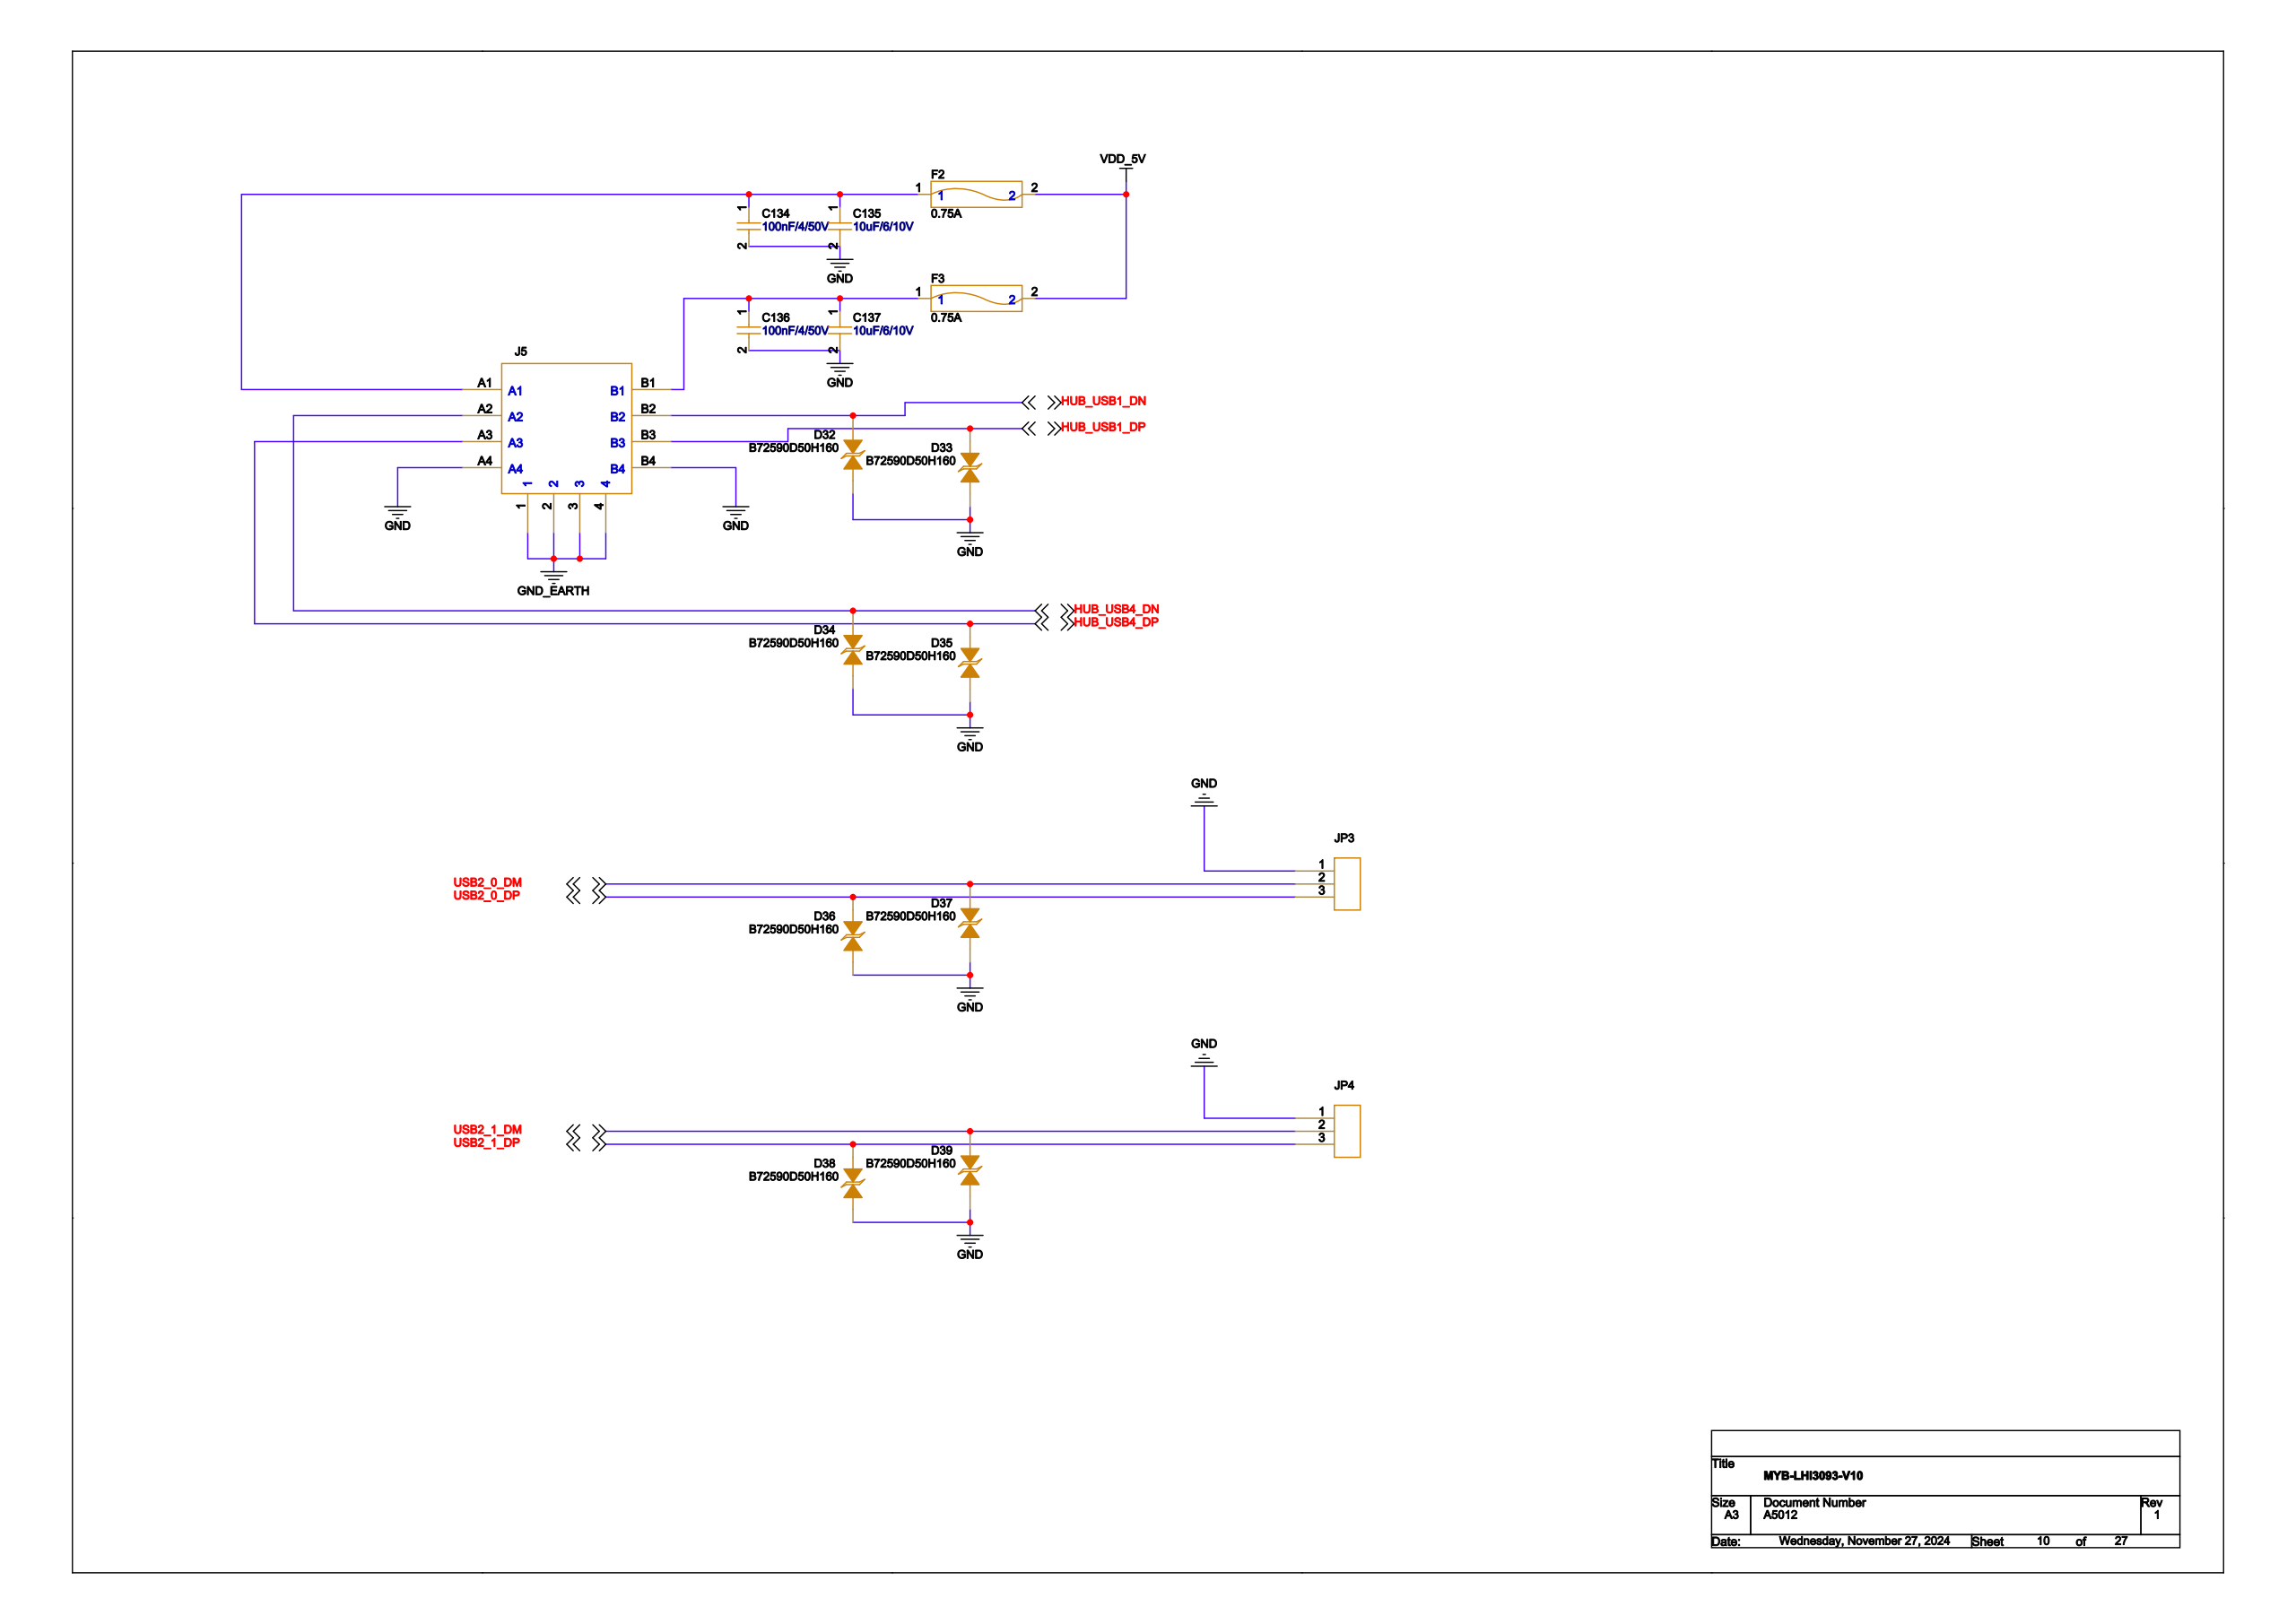Circuit board | Cadence Allegro | 1159 parts | 708 nets | one sheet of the schematic
Parts on this sheet (reference | value | footprint):
C134 | 100nF/4/50V | C0402
C135 | 10uF/6/10V | C0603
C136 | 100nF/4/50V | C0402
C137 | 10uF/6/10V | C0603
D32 | B72590D50H160 | D0402
D33 | B72590D50H160 | D0402
D34 | B72590D50H160 | D0402
D35 | B72590D50H160 | D0402
D36 | B72590D50H160 | D0402
D37 | B72590D50H160 | D0402
D38 | B72590D50H160 | D0402
D39 | B72590D50H160 | D0402
F2 | 0.75A | F1206
F3 | 0.75A | F1206
J5 | J5 | UB11121-8FDE-4F
JP3 | JP3 | CONN1X3-2_54-DIP
JP4 | JP3 | CONN1X3-2_54-DIP
Nets of these parts (net: part-pin ...):
GND: C134-2 C135-2 C136-2 C137-2 D32-1 D33-1 D34-1 D35-1 D36-1 D37-1 D38-1 D39-1 J5-A4 J5-B4 JP3-1 JP4-1
VDD_5V: F2-2 F3-2
N14871544: C134-1 C135-1 F2-1 J5-A1
N14871433: C136-1 C137-1 F3-1 J5-B1
GND_EARTH: J5-1 J5-2 J5-3 J5-4
HUB_USB1_DN: D32-2 J5-B2
HUB_USB1_DP: D33-2 J5-B3
HUB_USB4_DN: D34-2 J5-A2
HUB_USB4_DP: D35-2 J5-A3
USB2_0_DP: D36-2 JP3-3
USB2_0_DM: D37-2 JP3-2
USB2_1_DP: D38-2 JP4-3
USB2_1_DM: D39-2 JP4-2